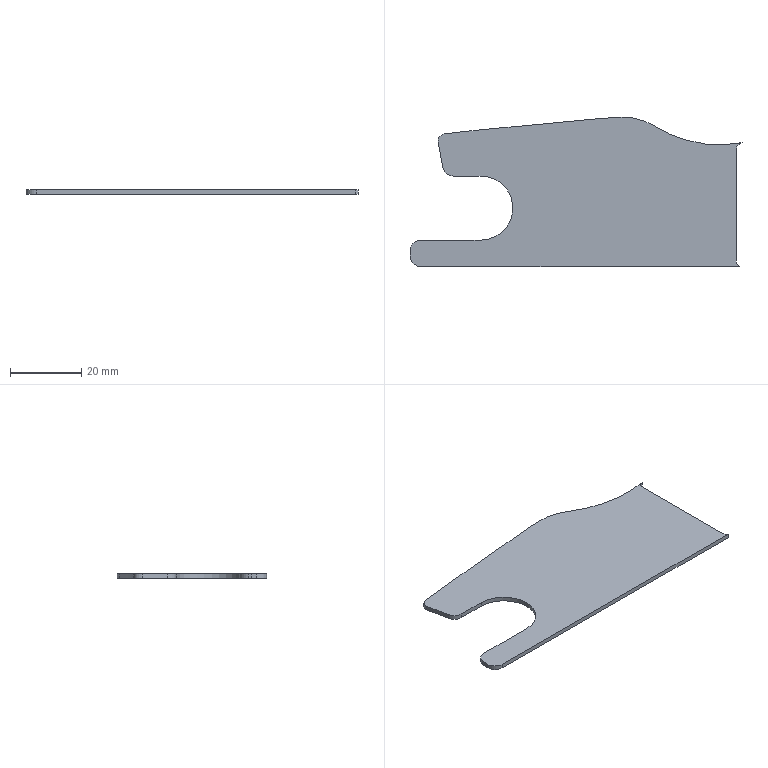Part | STEP file | gslz 2016.10.28-13_id242_x_t | 1 solid | 22 faces | box 93.462 x 42.065 x 1.25 mm | volume 3701 mm3 | plane 12 | cylinder 10 | commonest cylinder face diameters 4 x3 6 x3 18 x1 32 x1 68.841 x1 1089 x1